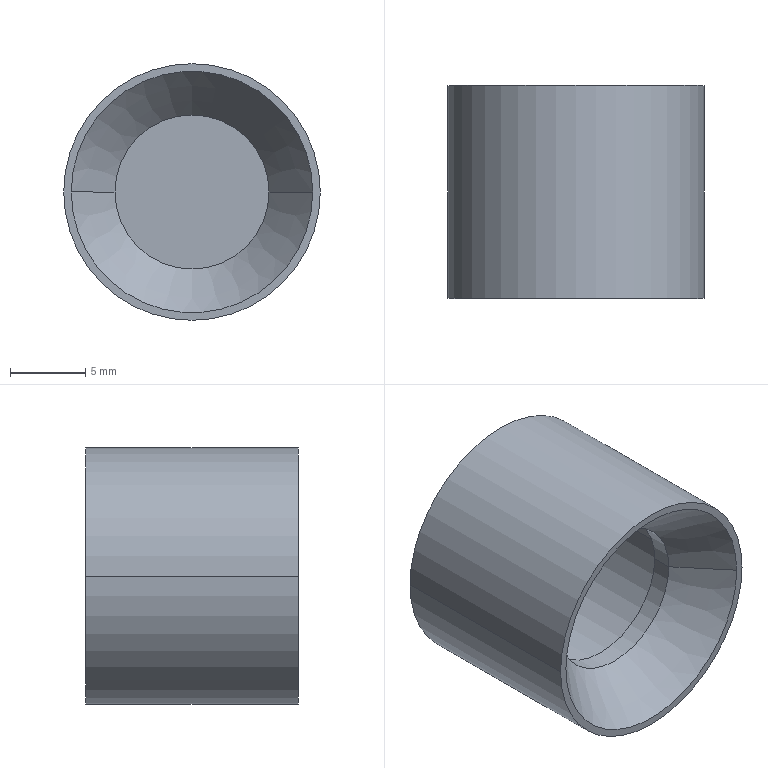Part | SolidWorks | features Revolution 1 | 1 solid | 12 faces | box 17 x 14.11 x 17 mm | volume 1515 mm3 | cylinder 6 | plane 4 | cone 2 | commonest cylinder face diameters 10.203 x2 13 x2 17 x2
STEP:
#1=CARTESIAN_POINT('',(5.102,3.344,0.));
#2=VERTEX_POINT('',#1);
#3=CARTESIAN_POINT('',(-5.102,3.344,0.));
#4=VERTEX_POINT('',#3);
#5=CARTESIAN_POINT('',(0.,3.344,0.));
#6=DIRECTION('',(0.,1.,0.));
#7=DIRECTION('',(-1.,0.,0.));
#8=AXIS2_PLACEMENT_3D('',#5,#6,#7);
#9=CIRCLE('',#8,5.102);
#10=EDGE_CURVE('',#2,#4,#9,.T.);
#11=ORIENTED_EDGE('',*,*,#10,.F.);
#12=CARTESIAN_POINT('',(5.102,4.666,0.));
#13=VERTEX_POINT('',#12);
#14=CARTESIAN_POINT('',(5.102,14.,0.));
#15=DIRECTION('',(0.,1.,0.));
#16=VECTOR('',#15,1000.);
#17=LINE('',#14,#16);
#18=EDGE_CURVE('',#2,#13,#17,.T.);
#19=ORIENTED_EDGE('',*,*,#18,.T.);
#20=CARTESIAN_POINT('',(-5.102,4.666,0.));
#21=VERTEX_POINT('',#20);
#22=CARTESIAN_POINT('',(0.,4.666,0.));
#23=DIRECTION('',(0.,1.,0.));
#24=DIRECTION('',(-1.,0.,0.));
#25=AXIS2_PLACEMENT_3D('',#22,#23,#24);
#26=CIRCLE('',#25,5.102);
#27=EDGE_CURVE('',#13,#21,#26,.T.);
#28=ORIENTED_EDGE('',*,*,#27,.T.);
#29=CARTESIAN_POINT('',(-5.102,14.,0.));
#30=DIRECTION('',(0.,1.,0.));
#31=VECTOR('',#30,1000.);
#32=LINE('',#29,#31);
#33=EDGE_CURVE('',#4,#21,#32,.T.);
#34=ORIENTED_EDGE('',*,*,#33,.F.);
#35=EDGE_LOOP('',(#11,#19,#28,#34));
#36=FACE_OUTER_BOUND('',#35,.T.);
#37=CARTESIAN_POINT('',(0.,14.,0.));
#38=DIRECTION('',(0.,1.,0.));
#39=DIRECTION('',(-1.,0.,0.));
#40=AXIS2_PLACEMENT_3D('',#37,#38,#39);
#41=CYLINDRICAL_SURFACE('',#40,5.102);
#42=ADVANCED_FACE('',(#36),#41,.F.);
#43=ORIENTED_EDGE('',*,*,#10,.T.);
#44=CARTESIAN_POINT('',(-8.,-0.11,0.));
#45=VERTEX_POINT('',#44);
#46=CARTESIAN_POINT('',(-8.,-0.11,0.));
#47=DIRECTION('',(-0.6428,-0.766,0.));
#48=VECTOR('',#47,1000.);
#49=LINE('',#46,#48);
#50=EDGE_CURVE('',#4,#45,#49,.T.);
#51=ORIENTED_EDGE('',*,*,#50,.T.);
#52=CARTESIAN_POINT('',(8.,-0.11,0.));
#53=VERTEX_POINT('',#52);
#54=CARTESIAN_POINT('',(0.,-0.11,0.));
#55=DIRECTION('',(0.,1.,0.));
#56=DIRECTION('',(-1.,0.,0.));
#57=AXIS2_PLACEMENT_3D('',#54,#55,#56);
#58=CIRCLE('',#57,8.);
#59=EDGE_CURVE('',#53,#45,#58,.T.);
#60=ORIENTED_EDGE('',*,*,#59,.F.);
#61=CARTESIAN_POINT('',(8.,-0.11,0.));
#62=DIRECTION('',(0.6428,-0.766,0.));
#63=VECTOR('',#62,1000.);
#64=LINE('',#61,#63);
#65=EDGE_CURVE('',#2,#53,#64,.T.);
#66=ORIENTED_EDGE('',*,*,#65,.F.);
#67=EDGE_LOOP('',(#43,#51,#60,#66));
#68=FACE_OUTER_BOUND('',#67,.T.);
#69=CARTESIAN_POINT('',(0.,-0.11,0.));
#70=DIRECTION('',(0.,-1.,0.));
#71=DIRECTION('',(1.,0.,0.));
#72=AXIS2_PLACEMENT_3D('',#69,#70,#71);
#73=CONICAL_SURFACE('',#72,8.,0.6981);
#74=ADVANCED_FACE('',(#68),#73,.F.);
#75=CARTESIAN_POINT('',(-8.5,-0.11,0.));
#76=VERTEX_POINT('',#75);
#77=CARTESIAN_POINT('',(8.5,-0.11,0.));
#78=VERTEX_POINT('',#77);
#79=CARTESIAN_POINT('',(0.,-0.11,0.));
#80=DIRECTION('',(0.,1.,0.));
#81=DIRECTION('',(-1.,0.,0.));
#82=AXIS2_PLACEMENT_3D('',#79,#80,#81);
#83=CIRCLE('',#82,8.5);
#84=EDGE_CURVE('',#76,#78,#83,.T.);
#85=ORIENTED_EDGE('',*,*,#84,.T.);
#86=CARTESIAN_POINT('',(8.5,14.,0.));
#87=VERTEX_POINT('',#86);
#88=CARTESIAN_POINT('',(8.5,14.,0.));
#89=DIRECTION('',(0.,1.,0.));
#90=VECTOR('',#89,1000.);
#91=LINE('',#88,#90);
#92=EDGE_CURVE('',#78,#87,#91,.T.);
#93=ORIENTED_EDGE('',*,*,#92,.T.);
#94=CARTESIAN_POINT('',(-8.5,14.,0.));
#95=VERTEX_POINT('',#94);
#96=CARTESIAN_POINT('',(0.,14.,0.));
#97=DIRECTION('',(0.,1.,0.));
#98=DIRECTION('',(-1.,0.,0.));
#99=AXIS2_PLACEMENT_3D('',#96,#97,#98);
#100=CIRCLE('',#99,8.5);
#101=EDGE_CURVE('',#95,#87,#100,.T.);
#102=ORIENTED_EDGE('',*,*,#101,.F.);
#103=CARTESIAN_POINT('',(-8.5,14.,0.));
#104=DIRECTION('',(0.,1.,0.));
#105=VECTOR('',#104,1000.);
#106=LINE('',#103,#105);
#107=EDGE_CURVE('',#76,#95,#106,.T.);
#108=ORIENTED_EDGE('',*,*,#107,.F.);
#109=EDGE_LOOP('',(#85,#93,#102,#108));
#110=FACE_OUTER_BOUND('',#109,.T.);
#111=CARTESIAN_POINT('',(0.,14.,0.));
#112=DIRECTION('',(0.,1.,0.));
#113=DIRECTION('',(-1.,0.,0.));
#114=AXIS2_PLACEMENT_3D('',#111,#112,#113);
#115=CYLINDRICAL_SURFACE('',#114,8.5);
#116=ADVANCED_FACE('',(#110),#115,.T.);
#117=CARTESIAN_POINT('',(6.5,4.666,0.));
#118=VERTEX_POINT('',#117);
#119=CARTESIAN_POINT('',(-6.5,4.666,0.));
#120=VERTEX_POINT('',#119);
#121=CARTESIAN_POINT('',(0.,4.666,0.));
#122=DIRECTION('',(0.,1.,0.));
#123=DIRECTION('',(-1.,0.,0.));
#124=AXIS2_PLACEMENT_3D('',#121,#122,#123);
#125=CIRCLE('',#124,6.5);
#126=EDGE_CURVE('',#118,#120,#125,.T.);
#127=ORIENTED_EDGE('',*,*,#126,.F.);
#128=CARTESIAN_POINT('',(6.5,13.,0.));
#129=VERTEX_POINT('',#128);
#130=CARTESIAN_POINT('',(6.5,14.,0.));
#131=DIRECTION('',(0.,1.,0.));
#132=VECTOR('',#131,1000.);
#133=LINE('',#130,#132);
#134=EDGE_CURVE('',#118,#129,#133,.T.);
#135=ORIENTED_EDGE('',*,*,#134,.T.);
#136=CARTESIAN_POINT('',(-6.5,13.,0.));
#137=VERTEX_POINT('',#136);
#138=CARTESIAN_POINT('',(0.,13.,0.));
#139=DIRECTION('',(0.,1.,0.));
#140=DIRECTION('',(-1.,0.,0.));
#141=AXIS2_PLACEMENT_3D('',#138,#139,#140);
#142=CIRCLE('',#141,6.5);
#143=EDGE_CURVE('',#129,#137,#142,.T.);
#144=ORIENTED_EDGE('',*,*,#143,.T.);
#145=CARTESIAN_POINT('',(-6.5,14.,0.));
#146=DIRECTION('',(0.,1.,0.));
#147=VECTOR('',#146,1000.);
#148=LINE('',#145,#147);
#149=EDGE_CURVE('',#120,#137,#148,.T.);
#150=ORIENTED_EDGE('',*,*,#149,.F.);
#151=EDGE_LOOP('',(#127,#135,#144,#150));
#152=FACE_OUTER_BOUND('',#151,.T.);
#153=CARTESIAN_POINT('',(0.,14.,0.));
#154=DIRECTION('',(0.,1.,0.));
#155=DIRECTION('',(-1.,0.,0.));
#156=AXIS2_PLACEMENT_3D('',#153,#154,#155);
#157=CYLINDRICAL_SURFACE('',#156,6.5);
#158=ADVANCED_FACE('',(#152),#157,.F.);
#159=ORIENTED_EDGE('',*,*,#134,.F.);
#160=CARTESIAN_POINT('',(0.,4.666,0.));
#161=DIRECTION('',(0.,1.,0.));
#162=DIRECTION('',(-1.,0.,0.));
#163=AXIS2_PLACEMENT_3D('',#160,#161,#162);
#164=CIRCLE('',#163,6.5);
#165=EDGE_CURVE('',#120,#118,#164,.T.);
#166=ORIENTED_EDGE('',*,*,#165,.F.);
#167=ORIENTED_EDGE('',*,*,#149,.T.);
#168=CARTESIAN_POINT('',(0.,13.,0.));
#169=DIRECTION('',(0.,1.,0.));
#170=DIRECTION('',(-1.,0.,0.));
#171=AXIS2_PLACEMENT_3D('',#168,#169,#170);
#172=CIRCLE('',#171,6.5);
#173=EDGE_CURVE('',#137,#129,#172,.T.);
#174=ORIENTED_EDGE('',*,*,#173,.T.);
#175=EDGE_LOOP('',(#159,#166,#167,#174));
#176=FACE_OUTER_BOUND('',#175,.T.);
#177=CARTESIAN_POINT('',(0.,14.,0.));
#178=DIRECTION('',(0.,1.,0.));
#179=DIRECTION('',(-1.,0.,0.));
#180=AXIS2_PLACEMENT_3D('',#177,#178,#179);
#181=CYLINDRICAL_SURFACE('',#180,6.5);
#182=ADVANCED_FACE('',(#176),#181,.F.);
#183=ORIENTED_EDGE('',*,*,#173,.F.);
#184=ORIENTED_EDGE('',*,*,#143,.F.);
#185=EDGE_LOOP('',(#183,#184));
#186=FACE_OUTER_BOUND('',#185,.T.);
#187=CARTESIAN_POINT('',(0.,13.,0.));
#188=DIRECTION('',(0.,-1.,0.));
#189=DIRECTION('',(1.,0.,0.));
#190=AXIS2_PLACEMENT_3D('',#187,#188,#189);
#191=PLANE('',#190);
#192=ADVANCED_FACE('',(#186),#191,.T.);
#193=ORIENTED_EDGE('',*,*,#101,.T.);
#194=CARTESIAN_POINT('',(0.,14.,0.));
#195=DIRECTION('',(0.,1.,0.));
#196=DIRECTION('',(-1.,0.,0.));
#197=AXIS2_PLACEMENT_3D('',#194,#195,#196);
#198=CIRCLE('',#197,8.5);
#199=EDGE_CURVE('',#87,#95,#198,.T.);
#200=ORIENTED_EDGE('',*,*,#199,.T.);
#201=EDGE_LOOP('',(#193,#200));
#202=FACE_OUTER_BOUND('',#201,.T.);
#203=CARTESIAN_POINT('',(0.,14.,0.));
#204=DIRECTION('',(0.,-1.,0.));
#205=DIRECTION('',(1.,0.,0.));
#206=AXIS2_PLACEMENT_3D('',#203,#204,#205);
#207=PLANE('',#206);
#208=ADVANCED_FACE('',(#202),#207,.F.);
#209=ORIENTED_EDGE('',*,*,#92,.F.);
#210=CARTESIAN_POINT('',(0.,-0.11,0.));
#211=DIRECTION('',(0.,1.,0.));
#212=DIRECTION('',(-1.,0.,0.));
#213=AXIS2_PLACEMENT_3D('',#210,#211,#212);
#214=CIRCLE('',#213,8.5);
#215=EDGE_CURVE('',#78,#76,#214,.T.);
#216=ORIENTED_EDGE('',*,*,#215,.T.);
#217=ORIENTED_EDGE('',*,*,#107,.T.);
#218=ORIENTED_EDGE('',*,*,#199,.F.);
#219=EDGE_LOOP('',(#209,#216,#217,#218));
#220=FACE_OUTER_BOUND('',#219,.T.);
#221=CARTESIAN_POINT('',(0.,14.,0.));
#222=DIRECTION('',(0.,1.,0.));
#223=DIRECTION('',(-1.,0.,0.));
#224=AXIS2_PLACEMENT_3D('',#221,#222,#223);
#225=CYLINDRICAL_SURFACE('',#224,8.5);
#226=ADVANCED_FACE('',(#220),#225,.T.);
#227=ORIENTED_EDGE('',*,*,#59,.T.);
#228=CARTESIAN_POINT('',(0.,-0.11,0.));
#229=DIRECTION('',(0.,1.,0.));
#230=DIRECTION('',(-1.,0.,0.));
#231=AXIS2_PLACEMENT_3D('',#228,#229,#230);
#232=CIRCLE('',#231,8.);
#233=EDGE_CURVE('',#45,#53,#232,.T.);
#234=ORIENTED_EDGE('',*,*,#233,.T.);
#235=EDGE_LOOP('',(#227,#234));
#236=FACE_BOUND('',#235,.T.);
#237=ORIENTED_EDGE('',*,*,#84,.F.);
#238=ORIENTED_EDGE('',*,*,#215,.F.);
#239=EDGE_LOOP('',(#237,#238));
#240=FACE_OUTER_BOUND('',#239,.T.);
#241=CARTESIAN_POINT('',(0.,-0.11,0.));
#242=DIRECTION('',(0.,-1.,0.));
#243=DIRECTION('',(1.,0.,0.));
#244=AXIS2_PLACEMENT_3D('',#241,#242,#243);
#245=PLANE('',#244);
#246=ADVANCED_FACE('',(#236,#240),#245,.T.);
#247=ORIENTED_EDGE('',*,*,#50,.F.);
#248=CARTESIAN_POINT('',(0.,3.344,0.));
#249=DIRECTION('',(0.,1.,0.));
#250=DIRECTION('',(-1.,0.,0.));
#251=AXIS2_PLACEMENT_3D('',#248,#249,#250);
#252=CIRCLE('',#251,5.102);
#253=EDGE_CURVE('',#4,#2,#252,.T.);
#254=ORIENTED_EDGE('',*,*,#253,.T.);
#255=ORIENTED_EDGE('',*,*,#65,.T.);
#256=ORIENTED_EDGE('',*,*,#233,.F.);
#257=EDGE_LOOP('',(#247,#254,#255,#256));
#258=FACE_OUTER_BOUND('',#257,.T.);
#259=CARTESIAN_POINT('',(0.,-0.11,0.));
#260=DIRECTION('',(0.,-1.,0.));
#261=DIRECTION('',(1.,0.,0.));
#262=AXIS2_PLACEMENT_3D('',#259,#260,#261);
#263=CONICAL_SURFACE('',#262,8.,0.6981);
#264=ADVANCED_FACE('',(#258),#263,.F.);
#265=ORIENTED_EDGE('',*,*,#18,.F.);
#266=ORIENTED_EDGE('',*,*,#253,.F.);
#267=ORIENTED_EDGE('',*,*,#33,.T.);
#268=CARTESIAN_POINT('',(0.,4.666,0.));
#269=DIRECTION('',(0.,1.,0.));
#270=DIRECTION('',(-1.,0.,0.));
#271=AXIS2_PLACEMENT_3D('',#268,#269,#270);
#272=CIRCLE('',#271,5.102);
#273=EDGE_CURVE('',#21,#13,#272,.T.);
#274=ORIENTED_EDGE('',*,*,#273,.T.);
#275=EDGE_LOOP('',(#265,#266,#267,#274));
#276=FACE_OUTER_BOUND('',#275,.T.);
#277=CARTESIAN_POINT('',(0.,14.,0.));
#278=DIRECTION('',(0.,1.,0.));
#279=DIRECTION('',(-1.,0.,0.));
#280=AXIS2_PLACEMENT_3D('',#277,#278,#279);
#281=CYLINDRICAL_SURFACE('',#280,5.102);
#282=ADVANCED_FACE('',(#276),#281,.F.);
#283=ORIENTED_EDGE('',*,*,#165,.T.);
#284=ORIENTED_EDGE('',*,*,#126,.T.);
#285=EDGE_LOOP('',(#283,#284));
#286=FACE_OUTER_BOUND('',#285,.T.);
#287=ORIENTED_EDGE('',*,*,#273,.F.);
#288=ORIENTED_EDGE('',*,*,#27,.F.);
#289=EDGE_LOOP('',(#287,#288));
#290=FACE_BOUND('',#289,.T.);
#291=CARTESIAN_POINT('',(0.,4.666,0.));
#292=DIRECTION('',(0.,1.,0.));
#293=DIRECTION('',(-1.,0.,0.));
#294=AXIS2_PLACEMENT_3D('',#291,#292,#293);
#295=PLANE('',#294);
#296=ADVANCED_FACE('',(#286,#290),#295,.T.);
#297=CLOSED_SHELL('',(#42,#74,#116,#158,#182,#192,#208,#226,#246,#264,#282,#296));
#298=MANIFOLD_SOLID_BREP('',#297);
#299=CARTESIAN_POINT('',(0.,0.,0.));
#300=DIRECTION('',(0.,0.,1.));
#301=DIRECTION('',(1.,0.,0.));
#302=AXIS2_PLACEMENT_3D('',#299,#300,#301);
#303=(LENGTH_UNIT()NAMED_UNIT(*)SI_UNIT(.MILLI.,.METRE.));
#304=UNCERTAINTY_MEASURE_WITH_UNIT(LENGTH_MEASURE(0.00001),#303,'','');
#305=(NAMED_UNIT(*)PLANE_ANGLE_UNIT()SI_UNIT($,.RADIAN.));
#306=(NAMED_UNIT(*)SI_UNIT($,.STERADIAN.)SOLID_ANGLE_UNIT());
#307=(GEOMETRIC_REPRESENTATION_CONTEXT(3)GLOBAL_UNCERTAINTY_ASSIGNED_CONTEXT((#304))GLOBAL_UNIT_ASSIGNED_CONTEXT((#303,#305,#306))REPRESENTATION_CONTEXT('',''));
#308=ADVANCED_BREP_SHAPE_REPRESENTATION('',(#298,#302),#307);